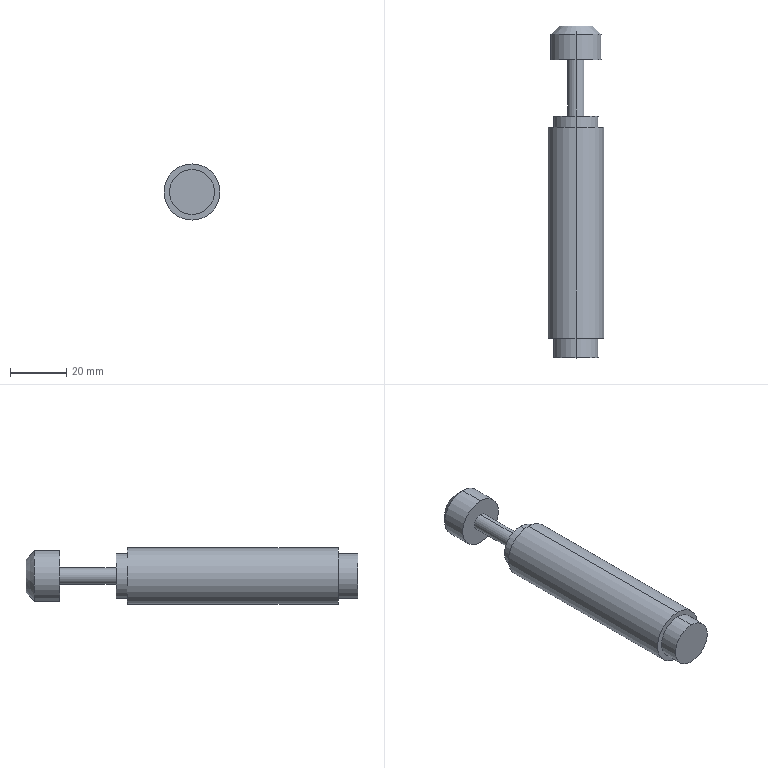Part | STEP file | PN_0009 (hydraulic changer ACA2020) | 1 solid | 18 faces | box 20 x 118 x 20 mm | volume 29167 mm3 | cylinder 10 | plane 6 | cone 2 | commonest cylinder face diameters 16 x4 6 x2 18 x2 20 x2
STEP:
#1=CARTESIAN_POINT('',(0.,0.,0.));
#2=DIRECTION('',(0.,0.,1.));
#3=DIRECTION('',(1.,0.,0.));
#4=AXIS2_PLACEMENT_3D('',#1,#2,#3);
#5=CARTESIAN_POINT('',(0.,118.,6.));
#6=VERTEX_POINT('',#5);
#7=CARTESIAN_POINT('',(0.,118.,-6.));
#8=VERTEX_POINT('',#7);
#9=CARTESIAN_POINT('',(0.,118.,0.));
#10=DIRECTION('',(0.,1.,0.));
#11=DIRECTION('',(0.,0.,1.));
#12=AXIS2_PLACEMENT_3D('',#9,#10,#11);
#13=CIRCLE('',#12,6.);
#14=CARTESIAN_POINT('',(0.,115.,0.));
#15=DIRECTION('',(0.,-1.,0.));
#16=DIRECTION('',(0.,0.,-1.));
#17=AXIS2_PLACEMENT_3D('',#14,#15,#16);
#18=CONICAL_SURFACE('',#17,9.,0.7854);
#19=CARTESIAN_POINT('',(3.142,-3.));
#20=DIRECTION('',(-1.,0.));
#21=VECTOR('',#20,1.);
#22=LINE('',#19,#21);
#23=(GEOMETRIC_REPRESENTATION_CONTEXT(2)PARAMETRIC_REPRESENTATION_CONTEXT()REPRESENTATION_CONTEXT('',''));
#24=DEFINITIONAL_REPRESENTATION('',(#22),#23);
#25=PCURVE('',#18,#24);
#26=CARTESIAN_POINT('',(9.,118.,0.));
#27=DIRECTION('',(0.,1.,0.));
#28=DIRECTION('',(0.,0.,1.));
#29=AXIS2_PLACEMENT_3D('',#26,#27,#28);
#30=PLANE('',#29);
#31=CARTESIAN_POINT('',(0.,-9.));
#32=DIRECTION('',(1.,0.));
#33=AXIS2_PLACEMENT_2D('',#31,#32);
#34=CIRCLE('',#33,6.);
#35=(GEOMETRIC_REPRESENTATION_CONTEXT(2)PARAMETRIC_REPRESENTATION_CONTEXT()REPRESENTATION_CONTEXT('',''));
#36=DEFINITIONAL_REPRESENTATION('',(#34),#35);
#37=PCURVE('',#30,#36);
#38=SURFACE_CURVE('',#13,(#25,#37),.PCURVE_S1.);
#39=EDGE_CURVE('',#6,#8,#38,.T.);
#40=ORIENTED_EDGE('',*,*,#39,.F.);
#41=CARTESIAN_POINT('',(0.,115.,9.));
#42=VERTEX_POINT('',#41);
#43=CARTESIAN_POINT('',(0.,115.,9.));
#44=DIRECTION('',(0.,-0.7071,0.7071));
#45=VECTOR('',#44,1.);
#46=LINE('',#43,#45);
#47=CARTESIAN_POINT('',(3.142,0.));
#48=DIRECTION('',(0.,1.));
#49=VECTOR('',#48,1.);
#50=LINE('',#47,#49);
#51=(GEOMETRIC_REPRESENTATION_CONTEXT(2)PARAMETRIC_REPRESENTATION_CONTEXT()REPRESENTATION_CONTEXT('',''));
#52=DEFINITIONAL_REPRESENTATION('',(#50),#51);
#53=PCURVE('',#18,#52);
#54=CARTESIAN_POINT('',(0.,115.,0.));
#55=DIRECTION('',(0.,-1.,0.));
#56=DIRECTION('',(0.,0.,-1.));
#57=AXIS2_PLACEMENT_3D('',#54,#55,#56);
#58=CONICAL_SURFACE('',#57,9.,0.7854);
#59=CARTESIAN_POINT('',(3.142,0.));
#60=DIRECTION('',(0.,1.));
#61=VECTOR('',#60,1.);
#62=LINE('',#59,#61);
#63=(GEOMETRIC_REPRESENTATION_CONTEXT(2)PARAMETRIC_REPRESENTATION_CONTEXT()REPRESENTATION_CONTEXT('',''));
#64=DEFINITIONAL_REPRESENTATION('',(#62),#63);
#65=PCURVE('',#58,#64);
#66=SURFACE_CURVE('',#46,(#53,#65),.PCURVE_S1.);
#67=EDGE_CURVE('',#6,#42,#66,.T.);
#68=ORIENTED_EDGE('',*,*,#67,.T.);
#69=CARTESIAN_POINT('',(0.,115.,-9.));
#70=VERTEX_POINT('',#69);
#71=CARTESIAN_POINT('',(0.,115.,0.));
#72=DIRECTION('',(0.,-1.,0.));
#73=DIRECTION('',(0.,0.,1.));
#74=AXIS2_PLACEMENT_3D('',#71,#72,#73);
#75=CIRCLE('',#74,9.);
#76=CARTESIAN_POINT('',(-3.142,0.));
#77=DIRECTION('',(1.,0.));
#78=VECTOR('',#77,1.);
#79=LINE('',#76,#78);
#80=(GEOMETRIC_REPRESENTATION_CONTEXT(2)PARAMETRIC_REPRESENTATION_CONTEXT()REPRESENTATION_CONTEXT('',''));
#81=DEFINITIONAL_REPRESENTATION('',(#79),#80);
#82=PCURVE('',#18,#81);
#83=CARTESIAN_POINT('',(0.,0.,0.));
#84=DIRECTION('',(0.,-1.,0.));
#85=DIRECTION('',(0.,0.,-1.));
#86=AXIS2_PLACEMENT_3D('',#83,#84,#85);
#87=CYLINDRICAL_SURFACE('',#86,9.);
#88=CARTESIAN_POINT('',(-3.142,-115.));
#89=DIRECTION('',(1.,0.));
#90=VECTOR('',#89,1.);
#91=LINE('',#88,#90);
#92=(GEOMETRIC_REPRESENTATION_CONTEXT(2)PARAMETRIC_REPRESENTATION_CONTEXT()REPRESENTATION_CONTEXT('',''));
#93=DEFINITIONAL_REPRESENTATION('',(#91),#92);
#94=PCURVE('',#87,#93);
#95=SURFACE_CURVE('',#75,(#82,#94),.PCURVE_S1.);
#96=EDGE_CURVE('',#70,#42,#95,.T.);
#97=ORIENTED_EDGE('',*,*,#96,.F.);
#98=CARTESIAN_POINT('',(0.,115.,-9.));
#99=DIRECTION('',(0.,-0.7071,-0.7071));
#100=VECTOR('',#99,1.);
#101=LINE('',#98,#100);
#102=CARTESIAN_POINT('',(0.,0.));
#103=DIRECTION('',(0.,1.));
#104=VECTOR('',#103,1.);
#105=LINE('',#102,#104);
#106=(GEOMETRIC_REPRESENTATION_CONTEXT(2)PARAMETRIC_REPRESENTATION_CONTEXT()REPRESENTATION_CONTEXT('',''));
#107=DEFINITIONAL_REPRESENTATION('',(#105),#106);
#108=PCURVE('',#18,#107);
#109=CARTESIAN_POINT('',(6.283,0.));
#110=DIRECTION('',(0.,1.));
#111=VECTOR('',#110,1.);
#112=LINE('',#109,#111);
#113=(GEOMETRIC_REPRESENTATION_CONTEXT(2)PARAMETRIC_REPRESENTATION_CONTEXT()REPRESENTATION_CONTEXT('',''));
#114=DEFINITIONAL_REPRESENTATION('',(#112),#113);
#115=PCURVE('',#58,#114);
#116=SURFACE_CURVE('',#101,(#108,#115),.PCURVE_S1.);
#117=EDGE_CURVE('',#8,#70,#116,.T.);
#118=ORIENTED_EDGE('',*,*,#117,.F.);
#119=EDGE_LOOP('',(#40,#68,#97,#118));
#120=FACE_BOUND('',#119,.T.);
#121=ADVANCED_FACE('',(#120),#18,.T.);
#122=ORIENTED_EDGE('',*,*,#96,.T.);
#123=CARTESIAN_POINT('',(0.,106.,9.));
#124=VERTEX_POINT('',#123);
#125=CARTESIAN_POINT('',(0.,0.,9.));
#126=DIRECTION('',(0.,-1.,0.));
#127=VECTOR('',#126,1.);
#128=LINE('',#125,#127);
#129=CARTESIAN_POINT('',(3.142,0.));
#130=DIRECTION('',(0.,1.));
#131=VECTOR('',#130,1.);
#132=LINE('',#129,#131);
#133=(GEOMETRIC_REPRESENTATION_CONTEXT(2)PARAMETRIC_REPRESENTATION_CONTEXT()REPRESENTATION_CONTEXT('',''));
#134=DEFINITIONAL_REPRESENTATION('',(#132),#133);
#135=PCURVE('',#87,#134);
#136=CARTESIAN_POINT('',(0.,0.,0.));
#137=DIRECTION('',(0.,-1.,0.));
#138=DIRECTION('',(0.,0.,-1.));
#139=AXIS2_PLACEMENT_3D('',#136,#137,#138);
#140=CYLINDRICAL_SURFACE('',#139,9.);
#141=CARTESIAN_POINT('',(3.142,0.));
#142=DIRECTION('',(0.,1.));
#143=VECTOR('',#142,1.);
#144=LINE('',#141,#143);
#145=(GEOMETRIC_REPRESENTATION_CONTEXT(2)PARAMETRIC_REPRESENTATION_CONTEXT()REPRESENTATION_CONTEXT('',''));
#146=DEFINITIONAL_REPRESENTATION('',(#144),#145);
#147=PCURVE('',#140,#146);
#148=SURFACE_CURVE('',#128,(#135,#147),.PCURVE_S1.);
#149=EDGE_CURVE('',#42,#124,#148,.T.);
#150=ORIENTED_EDGE('',*,*,#149,.T.);
#151=CARTESIAN_POINT('',(0.,106.,-9.));
#152=VERTEX_POINT('',#151);
#153=CARTESIAN_POINT('',(0.,106.,0.));
#154=DIRECTION('',(0.,-1.,0.));
#155=DIRECTION('',(0.,0.,-1.));
#156=AXIS2_PLACEMENT_3D('',#153,#154,#155);
#157=CIRCLE('',#156,9.);
#158=CARTESIAN_POINT('',(0.,-106.));
#159=DIRECTION('',(1.,0.));
#160=VECTOR('',#159,1.);
#161=LINE('',#158,#160);
#162=(GEOMETRIC_REPRESENTATION_CONTEXT(2)PARAMETRIC_REPRESENTATION_CONTEXT()REPRESENTATION_CONTEXT('',''));
#163=DEFINITIONAL_REPRESENTATION('',(#161),#162);
#164=PCURVE('',#87,#163);
#165=CARTESIAN_POINT('',(3.,106.,0.));
#166=DIRECTION('',(0.,-1.,0.));
#167=DIRECTION('',(0.,0.,-1.));
#168=AXIS2_PLACEMENT_3D('',#165,#166,#167);
#169=PLANE('',#168);
#170=CARTESIAN_POINT('',(0.,-3.));
#171=DIRECTION('',(1.,0.));
#172=AXIS2_PLACEMENT_2D('',#170,#171);
#173=CIRCLE('',#172,9.);
#174=(GEOMETRIC_REPRESENTATION_CONTEXT(2)PARAMETRIC_REPRESENTATION_CONTEXT()REPRESENTATION_CONTEXT('',''));
#175=DEFINITIONAL_REPRESENTATION('',(#173),#174);
#176=PCURVE('',#169,#175);
#177=SURFACE_CURVE('',#157,(#164,#176),.PCURVE_S1.);
#178=EDGE_CURVE('',#152,#124,#177,.T.);
#179=ORIENTED_EDGE('',*,*,#178,.F.);
#180=CARTESIAN_POINT('',(0.,0.,-9.));
#181=DIRECTION('',(0.,-1.,0.));
#182=VECTOR('',#181,1.);
#183=LINE('',#180,#182);
#184=CARTESIAN_POINT('',(0.,0.));
#185=DIRECTION('',(0.,1.));
#186=VECTOR('',#185,1.);
#187=LINE('',#184,#186);
#188=(GEOMETRIC_REPRESENTATION_CONTEXT(2)PARAMETRIC_REPRESENTATION_CONTEXT()REPRESENTATION_CONTEXT('',''));
#189=DEFINITIONAL_REPRESENTATION('',(#187),#188);
#190=PCURVE('',#87,#189);
#191=CARTESIAN_POINT('',(6.283,0.));
#192=DIRECTION('',(0.,1.));
#193=VECTOR('',#192,1.);
#194=LINE('',#191,#193);
#195=(GEOMETRIC_REPRESENTATION_CONTEXT(2)PARAMETRIC_REPRESENTATION_CONTEXT()REPRESENTATION_CONTEXT('',''));
#196=DEFINITIONAL_REPRESENTATION('',(#194),#195);
#197=PCURVE('',#140,#196);
#198=SURFACE_CURVE('',#183,(#190,#197),.PCURVE_S1.);
#199=EDGE_CURVE('',#70,#152,#198,.T.);
#200=ORIENTED_EDGE('',*,*,#199,.F.);
#201=EDGE_LOOP('',(#122,#150,#179,#200));
#202=FACE_BOUND('',#201,.T.);
#203=ADVANCED_FACE('',(#202),#87,.T.);
#204=CARTESIAN_POINT('',(0.,106.,-3.));
#205=VERTEX_POINT('',#204);
#206=CARTESIAN_POINT('',(0.,106.,3.));
#207=VERTEX_POINT('',#206);
#208=CARTESIAN_POINT('',(0.,106.,0.));
#209=DIRECTION('',(0.,-1.,0.));
#210=DIRECTION('',(0.,0.,-1.));
#211=AXIS2_PLACEMENT_3D('',#208,#209,#210);
#212=CIRCLE('',#211,3.);
#213=CARTESIAN_POINT('',(0.,0.,0.));
#214=DIRECTION('',(0.,-1.,0.));
#215=DIRECTION('',(0.,0.,-1.));
#216=AXIS2_PLACEMENT_3D('',#213,#214,#215);
#217=CYLINDRICAL_SURFACE('',#216,3.);
#218=CARTESIAN_POINT('',(0.,-106.));
#219=DIRECTION('',(1.,0.));
#220=VECTOR('',#219,1.);
#221=LINE('',#218,#220);
#222=(GEOMETRIC_REPRESENTATION_CONTEXT(2)PARAMETRIC_REPRESENTATION_CONTEXT()REPRESENTATION_CONTEXT('',''));
#223=DEFINITIONAL_REPRESENTATION('',(#221),#222);
#224=PCURVE('',#217,#223);
#225=CARTESIAN_POINT('',(0.,-3.));
#226=DIRECTION('',(1.,0.));
#227=AXIS2_PLACEMENT_2D('',#225,#226);
#228=CIRCLE('',#227,3.);
#229=(GEOMETRIC_REPRESENTATION_CONTEXT(2)PARAMETRIC_REPRESENTATION_CONTEXT()REPRESENTATION_CONTEXT('',''));
#230=DEFINITIONAL_REPRESENTATION('',(#228),#229);
#231=PCURVE('',#169,#230);
#232=SURFACE_CURVE('',#212,(#224,#231),.PCURVE_S1.);
#233=EDGE_CURVE('',#205,#207,#232,.T.);
#234=ORIENTED_EDGE('',*,*,#233,.T.);
#235=CARTESIAN_POINT('',(0.,86.,3.));
#236=VERTEX_POINT('',#235);
#237=CARTESIAN_POINT('',(0.,0.,3.));
#238=DIRECTION('',(0.,-1.,0.));
#239=VECTOR('',#238,1.);
#240=LINE('',#237,#239);
#241=CARTESIAN_POINT('',(3.142,0.));
#242=DIRECTION('',(0.,1.));
#243=VECTOR('',#242,1.);
#244=LINE('',#241,#243);
#245=(GEOMETRIC_REPRESENTATION_CONTEXT(2)PARAMETRIC_REPRESENTATION_CONTEXT()REPRESENTATION_CONTEXT('',''));
#246=DEFINITIONAL_REPRESENTATION('',(#244),#245);
#247=PCURVE('',#217,#246);
#248=CARTESIAN_POINT('',(0.,0.,0.));
#249=DIRECTION('',(0.,-1.,0.));
#250=DIRECTION('',(0.,0.,-1.));
#251=AXIS2_PLACEMENT_3D('',#248,#249,#250);
#252=CYLINDRICAL_SURFACE('',#251,3.);
#253=CARTESIAN_POINT('',(3.142,0.));
#254=DIRECTION('',(0.,1.));
#255=VECTOR('',#254,1.);
#256=LINE('',#253,#255);
#257=(GEOMETRIC_REPRESENTATION_CONTEXT(2)PARAMETRIC_REPRESENTATION_CONTEXT()REPRESENTATION_CONTEXT('',''));
#258=DEFINITIONAL_REPRESENTATION('',(#256),#257);
#259=PCURVE('',#252,#258);
#260=SURFACE_CURVE('',#240,(#247,#259),.PCURVE_S1.);
#261=EDGE_CURVE('',#207,#236,#260,.T.);
#262=ORIENTED_EDGE('',*,*,#261,.T.);
#263=CARTESIAN_POINT('',(0.,86.,-3.));
#264=VERTEX_POINT('',#263);
#265=CARTESIAN_POINT('',(0.,86.,0.));
#266=DIRECTION('',(0.,-1.,0.));
#267=DIRECTION('',(0.,0.,-1.));
#268=AXIS2_PLACEMENT_3D('',#265,#266,#267);
#269=CIRCLE('',#268,3.);
#270=CARTESIAN_POINT('',(0.,-86.));
#271=DIRECTION('',(1.,0.));
#272=VECTOR('',#271,1.);
#273=LINE('',#270,#272);
#274=(GEOMETRIC_REPRESENTATION_CONTEXT(2)PARAMETRIC_REPRESENTATION_CONTEXT()REPRESENTATION_CONTEXT('',''));
#275=DEFINITIONAL_REPRESENTATION('',(#273),#274);
#276=PCURVE('',#217,#275);
#277=CARTESIAN_POINT('',(8.,86.,0.));
#278=DIRECTION('',(0.,1.,0.));
#279=DIRECTION('',(0.,0.,1.));
#280=AXIS2_PLACEMENT_3D('',#277,#278,#279);
#281=PLANE('',#280);
#282=CARTESIAN_POINT('',(-3.,-8.));
#283=CARTESIAN_POINT('',(-3.,-2.804));
#284=CARTESIAN_POINT('',(1.5,-5.402));
#285=CARTESIAN_POINT('',(6.,-8.));
#286=CARTESIAN_POINT('',(1.5,-10.598));
#287=CARTESIAN_POINT('',(-3.,-13.196));
#288=CARTESIAN_POINT('',(-3.,-8.));
#289=(BOUNDED_CURVE()B_SPLINE_CURVE(2,(#282,#283,#284,#285,#286,#287,#288),.UNSPECIFIED.,.T.,.F.)B_SPLINE_CURVE_WITH_KNOTS((1,2,2,2,2,1),(-2.094,0.,2.094,4.189,6.283,8.378),.UNSPECIFIED.)CURVE()GEOMETRIC_REPRESENTATION_ITEM()RATIONAL_B_SPLINE_CURVE((1.,0.5,1.,0.5,1.,0.5,1.))REPRESENTATION_ITEM(''));
#290=(GEOMETRIC_REPRESENTATION_CONTEXT(2)PARAMETRIC_REPRESENTATION_CONTEXT()REPRESENTATION_CONTEXT('',''));
#291=DEFINITIONAL_REPRESENTATION('',(#289),#290);
#292=PCURVE('',#281,#291);
#293=SURFACE_CURVE('',#269,(#276,#292),.PCURVE_S1.);
#294=EDGE_CURVE('',#264,#236,#293,.T.);
#295=ORIENTED_EDGE('',*,*,#294,.F.);
#296=CARTESIAN_POINT('',(0.,0.,-3.));
#297=DIRECTION('',(0.,-1.,0.));
#298=VECTOR('',#297,1.);
#299=LINE('',#296,#298);
#300=CARTESIAN_POINT('',(0.,0.));
#301=DIRECTION('',(0.,1.));
#302=VECTOR('',#301,1.);
#303=LINE('',#300,#302);
#304=(GEOMETRIC_REPRESENTATION_CONTEXT(2)PARAMETRIC_REPRESENTATION_CONTEXT()REPRESENTATION_CONTEXT('',''));
#305=DEFINITIONAL_REPRESENTATION('',(#303),#304);
#306=PCURVE('',#217,#305);
#307=CARTESIAN_POINT('',(6.283,0.));
#308=DIRECTION('',(0.,1.));
#309=VECTOR('',#308,1.);
#310=LINE('',#307,#309);
#311=(GEOMETRIC_REPRESENTATION_CONTEXT(2)PARAMETRIC_REPRESENTATION_CONTEXT()REPRESENTATION_CONTEXT('',''));
#312=DEFINITIONAL_REPRESENTATION('',(#310),#311);
#313=PCURVE('',#252,#312);
#314=SURFACE_CURVE('',#299,(#306,#313),.PCURVE_S1.);
#315=EDGE_CURVE('',#205,#264,#314,.T.);
#316=ORIENTED_EDGE('',*,*,#315,.F.);
#317=EDGE_LOOP('',(#234,#262,#295,#316));
#318=FACE_BOUND('',#317,.T.);
#319=ADVANCED_FACE('',(#318),#217,.T.);
#320=CARTESIAN_POINT('',(0.,86.,-8.));
#321=VERTEX_POINT('',#320);
#322=CARTESIAN_POINT('',(0.,86.,8.));
#323=VERTEX_POINT('',#322);
#324=CARTESIAN_POINT('',(0.,86.,0.));
#325=DIRECTION('',(0.,-1.,0.));
#326=DIRECTION('',(0.,0.,-1.));
#327=AXIS2_PLACEMENT_3D('',#324,#325,#326);
#328=CIRCLE('',#327,8.);
#329=CARTESIAN_POINT('',(0.,0.,0.));
#330=DIRECTION('',(0.,-1.,0.));
#331=DIRECTION('',(0.,0.,-1.));
#332=AXIS2_PLACEMENT_3D('',#329,#330,#331);
#333=CYLINDRICAL_SURFACE('',#332,8.);
#334=CARTESIAN_POINT('',(0.,-86.));
#335=DIRECTION('',(1.,0.));
#336=VECTOR('',#335,1.);
#337=LINE('',#334,#336);
#338=(GEOMETRIC_REPRESENTATION_CONTEXT(2)PARAMETRIC_REPRESENTATION_CONTEXT()REPRESENTATION_CONTEXT('',''));
#339=DEFINITIONAL_REPRESENTATION('',(#337),#338);
#340=PCURVE('',#333,#339);
#341=CARTESIAN_POINT('',(-8.,-8.));
#342=CARTESIAN_POINT('',(-8.,5.856));
#343=CARTESIAN_POINT('',(4.,-1.072));
#344=CARTESIAN_POINT('',(16.,-8.));
#345=CARTESIAN_POINT('',(4.,-14.928));
#346=CARTESIAN_POINT('',(-8.,-21.856));
#347=CARTESIAN_POINT('',(-8.,-8.));
#348=(BOUNDED_CURVE()B_SPLINE_CURVE(2,(#341,#342,#343,#344,#345,#346,#347),.UNSPECIFIED.,.T.,.F.)B_SPLINE_CURVE_WITH_KNOTS((1,2,2,2,2,1),(-2.094,0.,2.094,4.189,6.283,8.378),.UNSPECIFIED.)CURVE()GEOMETRIC_REPRESENTATION_ITEM()RATIONAL_B_SPLINE_CURVE((1.,0.5,1.,0.5,1.,0.5,1.))REPRESENTATION_ITEM(''));
#349=(GEOMETRIC_REPRESENTATION_CONTEXT(2)PARAMETRIC_REPRESENTATION_CONTEXT()REPRESENTATION_CONTEXT('',''));
#350=DEFINITIONAL_REPRESENTATION('',(#348),#349);
#351=PCURVE('',#281,#350);
#352=SURFACE_CURVE('',#328,(#340,#351),.PCURVE_S1.);
#353=EDGE_CURVE('',#321,#323,#352,.T.);
#354=ORIENTED_EDGE('',*,*,#353,.T.);
#355=CARTESIAN_POINT('',(0.,82.,8.));
#356=VERTEX_POINT('',#355);
#357=CARTESIAN_POINT('',(0.,0.,8.));
#358=DIRECTION('',(0.,-1.,0.));
#359=VECTOR('',#358,1.);
#360=LINE('',#357,#359);
#361=CARTESIAN_POINT('',(3.142,0.));
#362=DIRECTION('',(0.,1.));
#363=VECTOR('',#362,1.);
#364=LINE('',#361,#363);
#365=(GEOMETRIC_REPRESENTATION_CONTEXT(2)PARAMETRIC_REPRESENTATION_CONTEXT()REPRESENTATION_CONTEXT('',''));
#366=DEFINITIONAL_REPRESENTATION('',(#364),#365);
#367=PCURVE('',#333,#366);
#368=CARTESIAN_POINT('',(0.,0.,0.));
#369=DIRECTION('',(0.,-1.,0.));
#370=DIRECTION('',(0.,0.,-1.));
#371=AXIS2_PLACEMENT_3D('',#368,#369,#370);
#372=CYLINDRICAL_SURFACE('',#371,8.);
#373=CARTESIAN_POINT('',(3.142,0.));
#374=DIRECTION('',(0.,1.));
#375=VECTOR('',#374,1.);
#376=LINE('',#373,#375);
#377=(GEOMETRIC_REPRESENTATION_CONTEXT(2)PARAMETRIC_REPRESENTATION_CONTEXT()REPRESENTATION_CONTEXT('',''));
#378=DEFINITIONAL_REPRESENTATION('',(#376),#377);
#379=PCURVE('',#372,#378);
#380=SURFACE_CURVE('',#360,(#367,#379),.PCURVE_S1.);
#381=EDGE_CURVE('',#323,#356,#380,.T.);
#382=ORIENTED_EDGE('',*,*,#381,.T.);
#383=CARTESIAN_POINT('',(0.,82.,-8.));
#384=VERTEX_POINT('',#383);
#385=CARTESIAN_POINT('',(0.,82.,0.));
#386=DIRECTION('',(0.,-1.,0.));
#387=DIRECTION('',(0.,0.,-1.));
#388=AXIS2_PLACEMENT_3D('',#385,#386,#387);
#389=CIRCLE('',#388,8.);
#390=CARTESIAN_POINT('',(0.,-82.));
#391=DIRECTION('',(1.,0.));
#392=VECTOR('',#391,1.);
#393=LINE('',#390,#392);
#394=(GEOMETRIC_REPRESENTATION_CONTEXT(2)PARAMETRIC_REPRESENTATION_CONTEXT()REPRESENTATION_CONTEXT('',''));
#395=DEFINITIONAL_REPRESENTATION('',(#393),#394);
#396=PCURVE('',#333,#395);
#397=CARTESIAN_POINT('',(10.,82.,0.));
#398=DIRECTION('',(0.,1.,0.));
#399=DIRECTION('',(0.,0.,1.));
#400=AXIS2_PLACEMENT_3D('',#397,#398,#399);
#401=PLANE('',#400);
#402=CARTESIAN_POINT('',(-8.,-10.));
#403=CARTESIAN_POINT('',(-8.,3.856));
#404=CARTESIAN_POINT('',(4.,-3.072));
#405=CARTESIAN_POINT('',(16.,-10.));
#406=CARTESIAN_POINT('',(4.,-16.928));
#407=CARTESIAN_POINT('',(-8.,-23.856));
#408=CARTESIAN_POINT('',(-8.,-10.));
#409=(BOUNDED_CURVE()B_SPLINE_CURVE(2,(#402,#403,#404,#405,#406,#407,#408),.UNSPECIFIED.,.T.,.F.)B_SPLINE_CURVE_WITH_KNOTS((1,2,2,2,2,1),(-2.094,0.,2.094,4.189,6.283,8.378),.UNSPECIFIED.)CURVE()GEOMETRIC_REPRESENTATION_ITEM()RATIONAL_B_SPLINE_CURVE((1.,0.5,1.,0.5,1.,0.5,1.))REPRESENTATION_ITEM(''));
#410=(GEOMETRIC_REPRESENTATION_CONTEXT(2)PARAMETRIC_REPRESENTATION_CONTEXT()REPRESENTATION_CONTEXT('',''));
#411=DEFINITIONAL_REPRESENTATION('',(#409),#410);
#412=PCURVE('',#401,#411);
#413=SURFACE_CURVE('',#389,(#396,#412),.PCURVE_S1.);
#414=EDGE_CURVE('',#384,#356,#413,.T.);
#415=ORIENTED_EDGE('',*,*,#414,.F.);
#416=CARTESIAN_POINT('',(0.,0.,-8.));
#417=DIRECTION('',(0.,-1.,0.));
#418=VECTOR('',#417,1.);
#419=LINE('',#416,#418);
#420=CARTESIAN_POINT('',(0.,0.));
#421=DIRECTION('',(0.,1.));
#422=VECTOR('',#421,1.);
#423=LINE('',#420,#422);
#424=(GEOMETRIC_REPRESENTATION_CONTEXT(2)PARAMETRIC_REPRESENTATION_CONTEXT()REPRESENTATION_CONTEXT('',''));
#425=DEFINITIONAL_REPRESENTATION('',(#423),#424);
#426=PCURVE('',#333,#425);
#427=CARTESIAN_POINT('',(6.283,0.));
#428=DIRECTION('',(0.,1.));
#429=VECTOR('',#428,1.);
#430=LINE('',#427,#429);
#431=(GEOMETRIC_REPRESENTATION_CONTEXT(2)PARAMETRIC_REPRESENTATION_CONTEXT()REPRESENTATION_CONTEXT('',''));
#432=DEFINITIONAL_REPRESENTATION('',(#430),#431);
#433=PCURVE('',#372,#432);
#434=SURFACE_CURVE('',#419,(#426,#433),.PCURVE_S1.);
#435=EDGE_CURVE('',#321,#384,#434,.T.);
#436=ORIENTED_EDGE('',*,*,#435,.F.);
#437=EDGE_LOOP('',(#354,#382,#415,#436));
#438=FACE_BOUND('',#437,.T.);
#439=ADVANCED_FACE('',(#438),#333,.T.);
#440=CARTESIAN_POINT('',(0.,82.,-10.));
#441=VERTEX_POINT('',#440);
#442=CARTESIAN_POINT('',(0.,82.,10.));
#443=VERTEX_POINT('',#442);
#444=CARTESIAN_POINT('',(0.,82.,0.));
#445=DIRECTION('',(0.,-1.,0.));
#446=DIRECTION('',(0.,0.,-1.));
#447=AXIS2_PLACEMENT_3D('',#444,#445,#446);
#448=CIRCLE('',#447,10.);
#449=CARTESIAN_POINT('',(0.,0.,0.));
#450=DIRECTION('',(0.,-1.,0.));
#451=DIRECTION('',(0.,0.,-1.));
#452=AXIS2_PLACEMENT_3D('',#449,#450,#451);
#453=CYLINDRICAL_SURFACE('',#452,10.);
#454=CARTESIAN_POINT('',(0.,-82.));
#455=DIRECTION('',(1.,0.));
#456=VECTOR('',#455,1.);
#457=LINE('',#454,#456);
#458=(GEOMETRIC_REPRESENTATION_CONTEXT(2)PARAMETRIC_REPRESENTATION_CONTEXT()REPRESENTATION_CONTEXT('',''));
#459=DEFINITIONAL_REPRESENTATION('',(#457),#458);
#460=PCURVE('',#453,#459);
#461=CARTESIAN_POINT('',(-10.,-10.));
#462=CARTESIAN_POINT('',(-10.,7.321));
#463=CARTESIAN_POINT('',(5.,-1.34));
#464=CARTESIAN_POINT('',(20.,-10.));
#465=CARTESIAN_POINT('',(5.,-18.66));
#466=CARTESIAN_POINT('',(-10.,-27.321));
#467=CARTESIAN_POINT('',(-10.,-10.));
#468=(BOUNDED_CURVE()B_SPLINE_CURVE(2,(#461,#462,#463,#464,#465,#466,#467),.UNSPECIFIED.,.T.,.F.)B_SPLINE_CURVE_WITH_KNOTS((1,2,2,2,2,1),(-2.094,0.,2.094,4.189,6.283,8.378),.UNSPECIFIED.)CURVE()GEOMETRIC_REPRESENTATION_ITEM()RATIONAL_B_SPLINE_CURVE((1.,0.5,1.,0.5,1.,0.5,1.))REPRESENTATION_ITEM(''));
#469=(GEOMETRIC_REPRESENTATION_CONTEXT(2)PARAMETRIC_REPRESENTATION_CONTEXT()REPRESENTATION_CONTEXT('',''));
#470=DEFINITIONAL_REPRESENTATION('',(#468),#469);
#471=PCURVE('',#401,#470);
#472=SURFACE_CURVE('',#448,(#460,#471),.PCURVE_S1.);
#473=EDGE_CURVE('',#441,#443,#472,.T.);
#474=ORIENTED_EDGE('',*,*,#473,.T.);
#475=CARTESIAN_POINT('',(0.,7.,10.));
#476=VERTEX_POINT('',#475);
#477=CARTESIAN_POINT('',(0.,0.,10.));
#478=DIRECTION('',(0.,-1.,0.));
#479=VECTOR('',#478,1.);
#480=LINE('',#477,#479);
#481=CARTESIAN_POINT('',(3.142,0.));
#482=DIRECTION('',(0.,1.));
#483=VECTOR('',#482,1.);
#484=LINE('',#481,#483);
#485=(GEOMETRIC_REPRESENTATION_CONTEXT(2)PARAMETRIC_REPRESENTATION_CONTEXT()REPRESENTATION_CONTEXT('',''));
#486=DEFINITIONAL_REPRESENTATION('',(#484),#485);
#487=PCURVE('',#453,#486);
#488=CARTESIAN_POINT('',(0.,0.,0.));
#489=DIRECTION('',(0.,-1.,0.));
#490=DIRECTION('',(0.,0.,-1.));
#491=AXIS2_PLACEMENT_3D('',#488,#489,#490);
#492=CYLINDRICAL_SURFACE('',#491,10.);
#493=CARTESIAN_POINT('',(3.142,0.));
#494=DIRECTION('',(0.,1.));
#495=VECTOR('',#494,1.);
#496=LINE('',#493,#495);
#497=(GEOMETRIC_REPRESENTATION_CONTEXT(2)PARAMETRIC_REPRESENTATION_CONTEXT()REPRESENTATION_CONTEXT('',''));
#498=DEFINITIONAL_REPRESENTATION('',(#496),#497);
#499=PCURVE('',#492,#498);
#500=SURFACE_CURVE('',#480,(#487,#499),.PCURVE_S1.);
#501=EDGE_CURVE('',#443,#476,#500,.T.);
#502=ORIENTED_EDGE('',*,*,#501,.T.);
#503=CARTESIAN_POINT('',(0.,7.,-10.));
#504=VERTEX_POINT('',#503);
#505=CARTESIAN_POINT('',(0.,7.,0.));
#506=DIRECTION('',(0.,-1.,0.));
#507=DIRECTION('',(0.,0.,-1.));
#508=AXIS2_PLACEMENT_3D('',#505,#506,#507);
#509=CIRCLE('',#508,10.);
#510=CARTESIAN_POINT('',(0.,-7.));
#511=DIRECTION('',(1.,0.));
#512=VECTOR('',#511,1.);
#513=LINE('',#510,#512);
#514=(GEOMETRIC_REPRESENTATION_CONTEXT(2)PARAMETRIC_REPRESENTATION_CONTEXT()REPRESENTATION_CONTEXT('',''));
#515=DEFINITIONAL_REPRESENTATION('',(#513),#514);
#516=PCURVE('',#453,#515);
#517=CARTESIAN_POINT('',(8.,7.,0.));
#518=DIRECTION('',(0.,-1.,0.));
#519=DIRECTION('',(0.,0.,-1.));
#520=AXIS2_PLACEMENT_3D('',#517,#518,#519);
#521=PLANE('',#520);
#522=CARTESIAN_POINT('',(0.,-8.));
#523=DIRECTION('',(1.,0.));
#524=AXIS2_PLACEMENT_2D('',#522,#523);
#525=CIRCLE('',#524,10.);
#526=(GEOMETRIC_REPRESENTATION_CONTEXT(2)PARAMETRIC_REPRESENTATION_CONTEXT()REPRESENTATION_CONTEXT('',''));
#527=DEFINITIONAL_REPRESENTATION('',(#525),#526);
#528=PCURVE('',#521,#527);
#529=SURFACE_CURVE('',#509,(#516,#528),.PCURVE_S1.);
#530=EDGE_CURVE('',#504,#476,#529,.T.);
#531=ORIENTED_EDGE('',*,*,#530,.F.);
#532=CARTESIAN_POINT('',(0.,0.,-10.));
#533=DIRECTION('',(0.,-1.,0.));
#534=VECTOR('',#533,1.);
#535=LINE('',#532,#534);
#536=CARTESIAN_POINT('',(0.,0.));
#537=DIRECTION('',(0.,1.));
#538=VECTOR('',#537,1.);
#539=LINE('',#536,#538);
#540=(GEOMETRIC_REPRESENTATION_CONTEXT(2)PARAMETRIC_REPRESENTATION_CONTEXT()REPRESENTATION_CONTEXT('',''));
#541=DEFINITIONAL_REPRESENTATION('',(#539),#540);
#542=PCURVE('',#453,#541);
#543=CARTESIAN_POINT('',(6.283,0.));
#544=DIRECTION('',(0.,1.));
#545=VECTOR('',#544,1.);
#546=LINE('',#543,#545);
#547=(GEOMETRIC_REPRESENTATION_CONTEXT(2)PARAMETRIC_REPRESENTATION_CONTEXT()REPRESENTATION_CONTEXT('',''));
#548=DEFINITIONAL_REPRESENTATION('',(#546),#547);
#549=PCURVE('',#492,#548);
#550=SURFACE_CURVE('',#535,(#542,#549),.PCURVE_S1.);
#551=EDGE_CURVE('',#441,#504,#550,.T.);
#552=ORIENTED_EDGE('',*,*,#551,.F.);
#553=EDGE_LOOP('',(#474,#502,#531,#552));
#554=FACE_BOUND('',#553,.T.);
#555=ADVANCED_FACE('',(#554),#453,.T.);
#556=CARTESIAN_POINT('',(0.,7.,-8.));
#557=VERTEX_POINT('',#556);
#558=CARTESIAN_POINT('',(0.,7.,8.));
#559=VERTEX_POINT('',#558);
#560=CARTESIAN_POINT('',(0.,7.,0.));
#561=DIRECTION('',(0.,-1.,0.));
#562=DIRECTION('',(0.,0.,-1.));
#563=AXIS2_PLACEMENT_3D('',#560,#561,#562);
#564=CIRCLE('',#563,8.);
#565=CARTESIAN_POINT('',(0.,0.,0.));
#566=DIRECTION('',(0.,-1.,0.));
#567=DIRECTION('',(0.,0.,-1.));
#568=AXIS2_PLACEMENT_3D('',#565,#566,#567);
#569=CYLINDRICAL_SURFACE('',#568,8.);
#570=CARTESIAN_POINT('',(0.,-7.));
#571=DIRECTION('',(1.,0.));
#572=VECTOR('',#571,1.);
#573=LINE('',#570,#572);
#574=(GEOMETRIC_REPRESENTATION_CONTEXT(2)PARAMETRIC_REPRESENTATION_CONTEXT()REPRESENTATION_CONTEXT('',''));
#575=DEFINITIONAL_REPRESENTATION('',(#573),#574);
#576=PCURVE('',#569,#575);
#577=CARTESIAN_POINT('',(0.,-8.));
#578=DIRECTION('',(1.,0.));
#579=AXIS2_PLACEMENT_2D('',#577,#578);
#580=CIRCLE('',#579,8.);
#581=(GEOMETRIC_REPRESENTATION_CONTEXT(2)PARAMETRIC_REPRESENTATION_CONTEXT()REPRESENTATION_CONTEXT('',''));
#582=DEFINITIONAL_REPRESENTATION('',(#580),#581);
#583=PCURVE('',#521,#582);
#584=SURFACE_CURVE('',#564,(#576,#583),.PCURVE_S1.);
#585=EDGE_CURVE('',#557,#559,#584,.T.);
#586=ORIENTED_EDGE('',*,*,#585,.T.);
#587=CARTESIAN_POINT('',(0.,0.,8.));
#588=VERTEX_POINT('',#587);
#589=CARTESIAN_POINT('',(0.,0.,8.));
#590=DIRECTION('',(0.,-1.,0.));
#591=VECTOR('',#590,1.);
#592=LINE('',#589,#591);
#593=CARTESIAN_POINT('',(3.142,0.));
#594=DIRECTION('',(0.,1.));
#595=VECTOR('',#594,1.);
#596=LINE('',#593,#595);
#597=(GEOMETRIC_REPRESENTATION_CONTEXT(2)PARAMETRIC_REPRESENTATION_CONTEXT()REPRESENTATION_CONTEXT('',''));
#598=DEFINITIONAL_REPRESENTATION('',(#596),#597);
#599=PCURVE('',#569,#598);
#600=CARTESIAN_POINT('',(0.,0.,0.));
#601=DIRECTION('',(0.,-1.,0.));
#602=DIRECTION('',(0.,0.,-1.));
#603=AXIS2_PLACEMENT_3D('',#600,#601,#602);
#604=CYLINDRICAL_SURFACE('',#603,8.);
#605=CARTESIAN_POINT('',(3.142,0.));
#606=DIRECTION('',(0.,1.));
#607=VECTOR('',#606,1.);
#608=LINE('',#605,#607);
#609=(GEOMETRIC_REPRESENTATION_CONTEXT(2)PARAMETRIC_REPRESENTATION_CONTEXT()REPRESENTATION_CONTEXT('',''));
#610=DEFINITIONAL_REPRESENTATION('',(#608),#609);
#611=PCURVE('',#604,#610);
#612=SURFACE_CURVE('',#592,(#599,#611),.PCURVE_S1.);
#613=EDGE_CURVE('',#559,#588,#612,.T.);
#614=ORIENTED_EDGE('',*,*,#613,.T.);
#615=CARTESIAN_POINT('',(0.,0.,-8.));
#616=VERTEX_POINT('',#615);
#617=CARTESIAN_POINT('',(0.,0.,0.));
#618=DIRECTION('',(0.,-1.,0.));
#619=DIRECTION('',(0.,0.,-1.));
#620=AXIS2_PLACEMENT_3D('',#617,#618,#619);
#621=CIRCLE('',#620,8.);
#622=CARTESIAN_POINT('',(0.,0.));
#623=DIRECTION('',(1.,0.));
#624=VECTOR('',#623,1.);
#625=LINE('',#622,#624);
#626=(GEOMETRIC_REPRESENTATION_CONTEXT(2)PARAMETRIC_REPRESENTATION_CONTEXT()REPRESENTATION_CONTEXT('',''));
#627=DEFINITIONAL_REPRESENTATION('',(#625),#626);
#628=PCURVE('',#569,#627);
#629=CARTESIAN_POINT('',(0.,0.,0.));
#630=DIRECTION('',(0.,-1.,0.));
#631=DIRECTION('',(0.,0.,-1.));
#632=AXIS2_PLACEMENT_3D('',#629,#630,#631);
#633=PLANE('',#632);
#634=CARTESIAN_POINT('',(0.,0.));
#635=DIRECTION('',(1.,0.));
#636=AXIS2_PLACEMENT_2D('',#634,#635);
#637=CIRCLE('',#636,8.);
#638=(GEOMETRIC_REPRESENTATION_CONTEXT(2)PARAMETRIC_REPRESENTATION_CONTEXT()REPRESENTATION_CONTEXT('',''));
#639=DEFINITIONAL_REPRESENTATION('',(#637),#638);
#640=PCURVE('',#633,#639);
#641=SURFACE_CURVE('',#621,(#628,#640),.PCURVE_S1.);
#642=EDGE_CURVE('',#616,#588,#641,.T.);
#643=ORIENTED_EDGE('',*,*,#642,.F.);
#644=CARTESIAN_POINT('',(0.,0.,-8.));
#645=DIRECTION('',(0.,-1.,0.));
#646=VECTOR('',#645,1.);
#647=LINE('',#644,#646);
#648=CARTESIAN_POINT('',(0.,0.));
#649=DIRECTION('',(0.,1.));
#650=VECTOR('',#649,1.);
#651=LINE('',#648,#650);
#652=(GEOMETRIC_REPRESENTATION_CONTEXT(2)PARAMETRIC_REPRESENTATION_CONTEXT()REPRESENTATION_CONTEXT('',''));
#653=DEFINITIONAL_REPRESENTATION('',(#651),#652);
#654=PCURVE('',#569,#653);
#655=CARTESIAN_POINT('',(6.283,0.));
#656=DIRECTION('',(0.,1.));
#657=VECTOR('',#656,1.);
#658=LINE('',#655,#657);
#659=(GEOMETRIC_REPRESENTATION_CONTEXT(2)PARAMETRIC_REPRESENTATION_CONTEXT()REPRESENTATION_CONTEXT('',''));
#660=DEFINITIONAL_REPRESENTATION('',(#658),#659);
#661=PCURVE('',#604,#660);
#662=SURFACE_CURVE('',#647,(#654,#661),.PCURVE_S1.);
#663=EDGE_CURVE('',#557,#616,#662,.T.);
#664=ORIENTED_EDGE('',*,*,#663,.F.);
#665=EDGE_LOOP('',(#586,#614,#643,#664));
#666=FACE_BOUND('',#665,.T.);
#667=ADVANCED_FACE('',(#666),#569,.T.);
#668=ORIENTED_EDGE('',*,*,#642,.T.);
#669=CARTESIAN_POINT('',(0.,0.,0.));
#670=DIRECTION('',(0.,-1.,0.));
#671=DIRECTION('',(0.,0.,-1.));
#672=AXIS2_PLACEMENT_3D('',#669,#670,#671);
#673=CIRCLE('',#672,8.);
#674=CARTESIAN_POINT('',(0.,0.));
#675=DIRECTION('',(1.,0.));
#676=AXIS2_PLACEMENT_2D('',#674,#675);
#677=CIRCLE('',#676,8.);
#678=(GEOMETRIC_REPRESENTATION_CONTEXT(2)PARAMETRIC_REPRESENTATION_CONTEXT()REPRESENTATION_CONTEXT('',''));
#679=DEFINITIONAL_REPRESENTATION('',(#677),#678);
#680=PCURVE('',#633,#679);
#681=CARTESIAN_POINT('',(0.,0.));
#682=DIRECTION('',(1.,0.));
#683=VECTOR('',#682,1.);
#684=LINE('',#681,#683);
#685=(GEOMETRIC_REPRESENTATION_CONTEXT(2)PARAMETRIC_REPRESENTATION_CONTEXT()REPRESENTATION_CONTEXT('',''));
#686=DEFINITIONAL_REPRESENTATION('',(#684),#685);
#687=PCURVE('',#604,#686);
#688=SURFACE_CURVE('',#673,(#680,#687),.PCURVE_S1.);
#689=EDGE_CURVE('',#588,#616,#688,.T.);
#690=ORIENTED_EDGE('',*,*,#689,.T.);
#691=EDGE_LOOP('',(#668,#690));
#692=FACE_BOUND('',#691,.T.);
#693=ADVANCED_FACE('',(#692),#633,.T.);
#694=ORIENTED_EDGE('',*,*,#613,.F.);
#695=CARTESIAN_POINT('',(0.,7.,0.));
#696=DIRECTION('',(0.,-1.,0.));
#697=DIRECTION('',(0.,0.,-1.));
#698=AXIS2_PLACEMENT_3D('',#695,#696,#697);
#699=CIRCLE('',#698,8.);
#700=CARTESIAN_POINT('',(0.,-7.));
#701=DIRECTION('',(1.,0.));
#702=VECTOR('',#701,1.);
#703=LINE('',#700,#702);
#704=(GEOMETRIC_REPRESENTATION_CONTEXT(2)PARAMETRIC_REPRESENTATION_CONTEXT()REPRESENTATION_CONTEXT('',''));
#705=DEFINITIONAL_REPRESENTATION('',(#703),#704);
#706=PCURVE('',#604,#705);
#707=CARTESIAN_POINT('',(0.,-8.));
#708=DIRECTION('',(1.,0.));
#709=AXIS2_PLACEMENT_2D('',#707,#708);
#710=CIRCLE('',#709,8.);
#711=(GEOMETRIC_REPRESENTATION_CONTEXT(2)PARAMETRIC_REPRESENTATION_CONTEXT()REPRESENTATION_CONTEXT('',''));
#712=DEFINITIONAL_REPRESENTATION('',(#710),#711);
#713=PCURVE('',#521,#712);
#714=SURFACE_CURVE('',#699,(#706,#713),.PCURVE_S1.);
#715=EDGE_CURVE('',#559,#557,#714,.T.);
#716=ORIENTED_EDGE('',*,*,#715,.T.);
#717=ORIENTED_EDGE('',*,*,#663,.T.);
#718=ORIENTED_EDGE('',*,*,#689,.F.);
#719=EDGE_LOOP('',(#694,#716,#717,#718));
#720=FACE_BOUND('',#719,.T.);
#721=ADVANCED_FACE('',(#720),#604,.T.);
#722=ORIENTED_EDGE('',*,*,#530,.T.);
#723=CARTESIAN_POINT('',(0.,7.,0.));
#724=DIRECTION('',(0.,-1.,0.));
#725=DIRECTION('',(0.,0.,-1.));
#726=AXIS2_PLACEMENT_3D('',#723,#724,#725);
#727=CIRCLE('',#726,10.);
#728=CARTESIAN_POINT('',(0.,-8.));
#729=DIRECTION('',(1.,0.));
#730=AXIS2_PLACEMENT_2D('',#728,#729);
#731=CIRCLE('',#730,10.);
#732=(GEOMETRIC_REPRESENTATION_CONTEXT(2)PARAMETRIC_REPRESENTATION_CONTEXT()REPRESENTATION_CONTEXT('',''));
#733=DEFINITIONAL_REPRESENTATION('',(#731),#732);
#734=PCURVE('',#521,#733);
#735=CARTESIAN_POINT('',(0.,-7.));
#736=DIRECTION('',(1.,0.));
#737=VECTOR('',#736,1.);
#738=LINE('',#735,#737);
#739=(GEOMETRIC_REPRESENTATION_CONTEXT(2)PARAMETRIC_REPRESENTATION_CONTEXT()REPRESENTATION_CONTEXT('',''));
#740=DEFINITIONAL_REPRESENTATION('',(#738),#739);
#741=PCURVE('',#492,#740);
#742=SURFACE_CURVE('',#727,(#734,#741),.PCURVE_S1.);
#743=EDGE_CURVE('',#476,#504,#742,.T.);
#744=ORIENTED_EDGE('',*,*,#743,.T.);
#745=EDGE_LOOP('',(#722,#744));
#746=FACE_BOUND('',#745,.T.);
#747=ORIENTED_EDGE('',*,*,#585,.F.);
#748=ORIENTED_EDGE('',*,*,#715,.F.);
#749=EDGE_LOOP('',(#747,#748));
#750=FACE_BOUND('',#749,.T.);
#751=ADVANCED_FACE('',(#746,#750),#521,.T.);
#752=ORIENTED_EDGE('',*,*,#501,.F.);
#753=CARTESIAN_POINT('',(0.,82.,0.));
#754=DIRECTION('',(0.,-1.,0.));
#755=DIRECTION('',(0.,0.,-1.));
#756=AXIS2_PLACEMENT_3D('',#753,#754,#755);
#757=CIRCLE('',#756,10.);
#758=CARTESIAN_POINT('',(0.,-82.));
#759=DIRECTION('',(1.,0.));
#760=VECTOR('',#759,1.);
#761=LINE('',#758,#760);
#762=(GEOMETRIC_REPRESENTATION_CONTEXT(2)PARAMETRIC_REPRESENTATION_CONTEXT()REPRESENTATION_CONTEXT('',''));
#763=DEFINITIONAL_REPRESENTATION('',(#761),#762);
#764=PCURVE('',#492,#763);
#765=CARTESIAN_POINT('',(-10.,-10.));
#766=CARTESIAN_POINT('',(-10.,7.321));
#767=CARTESIAN_POINT('',(5.,-1.34));
#768=CARTESIAN_POINT('',(20.,-10.));
#769=CARTESIAN_POINT('',(5.,-18.66));
#770=CARTESIAN_POINT('',(-10.,-27.321));
#771=CARTESIAN_POINT('',(-10.,-10.));
#772=(BOUNDED_CURVE()B_SPLINE_CURVE(2,(#765,#766,#767,#768,#769,#770,#771),.UNSPECIFIED.,.T.,.F.)B_SPLINE_CURVE_WITH_KNOTS((1,2,2,2,2,1),(-2.094,0.,2.094,4.189,6.283,8.378),.UNSPECIFIED.)CURVE()GEOMETRIC_REPRESENTATION_ITEM()RATIONAL_B_SPLINE_CURVE((1.,0.5,1.,0.5,1.,0.5,1.))REPRESENTATION_ITEM(''));
#773=(GEOMETRIC_REPRESENTATION_CONTEXT(2)PARAMETRIC_REPRESENTATION_CONTEXT()REPRESENTATION_CONTEXT('',''));
#774=DEFINITIONAL_REPRESENTATION('',(#772),#773);
#775=PCURVE('',#401,#774);
#776=SURFACE_CURVE('',#757,(#764,#775),.PCURVE_S1.);
#777=EDGE_CURVE('',#443,#441,#776,.T.);
#778=ORIENTED_EDGE('',*,*,#777,.T.);
#779=ORIENTED_EDGE('',*,*,#551,.T.);
#780=ORIENTED_EDGE('',*,*,#743,.F.);
#781=EDGE_LOOP('',(#752,#778,#779,#780));
#782=FACE_BOUND('',#781,.T.);
#783=ADVANCED_FACE('',(#782),#492,.T.);
#784=ORIENTED_EDGE('',*,*,#414,.T.);
#785=CARTESIAN_POINT('',(0.,82.,0.));
#786=DIRECTION('',(0.,-1.,0.));
#787=DIRECTION('',(0.,0.,-1.));
#788=AXIS2_PLACEMENT_3D('',#785,#786,#787);
#789=CIRCLE('',#788,8.);
#790=CARTESIAN_POINT('',(-8.,-10.));
#791=CARTESIAN_POINT('',(-8.,3.856));
#792=CARTESIAN_POINT('',(4.,-3.072));
#793=CARTESIAN_POINT('',(16.,-10.));
#794=CARTESIAN_POINT('',(4.,-16.928));
#795=CARTESIAN_POINT('',(-8.,-23.856));
#796=CARTESIAN_POINT('',(-8.,-10.));
#797=(BOUNDED_CURVE()B_SPLINE_CURVE(2,(#790,#791,#792,#793,#794,#795,#796),.UNSPECIFIED.,.T.,.F.)B_SPLINE_CURVE_WITH_KNOTS((1,2,2,2,2,1),(-2.094,0.,2.094,4.189,6.283,8.378),.UNSPECIFIED.)CURVE()GEOMETRIC_REPRESENTATION_ITEM()RATIONAL_B_SPLINE_CURVE((1.,0.5,1.,0.5,1.,0.5,1.))REPRESENTATION_ITEM(''));
#798=(GEOMETRIC_REPRESENTATION_CONTEXT(2)PARAMETRIC_REPRESENTATION_CONTEXT()REPRESENTATION_CONTEXT('',''));
#799=DEFINITIONAL_REPRESENTATION('',(#797),#798);
#800=PCURVE('',#401,#799);
#801=CARTESIAN_POINT('',(0.,-82.));
#802=DIRECTION('',(1.,0.));
#803=VECTOR('',#802,1.);
#804=LINE('',#801,#803);
#805=(GEOMETRIC_REPRESENTATION_CONTEXT(2)PARAMETRIC_REPRESENTATION_CONTEXT()REPRESENTATION_CONTEXT('',''));
#806=DEFINITIONAL_REPRESENTATION('',(#804),#805);
#807=PCURVE('',#372,#806);
#808=SURFACE_CURVE('',#789,(#800,#807),.PCURVE_S1.);
#809=EDGE_CURVE('',#356,#384,#808,.T.);
#810=ORIENTED_EDGE('',*,*,#809,.T.);
#811=EDGE_LOOP('',(#784,#810));
#812=FACE_BOUND('',#811,.T.);
#813=ORIENTED_EDGE('',*,*,#473,.F.);
#814=ORIENTED_EDGE('',*,*,#777,.F.);
#815=EDGE_LOOP('',(#813,#814));
#816=FACE_BOUND('',#815,.T.);
#817=ADVANCED_FACE('',(#812,#816),#401,.T.);
#818=ORIENTED_EDGE('',*,*,#381,.F.);
#819=CARTESIAN_POINT('',(0.,86.,0.));
#820=DIRECTION('',(0.,-1.,0.));
#821=DIRECTION('',(0.,0.,-1.));
#822=AXIS2_PLACEMENT_3D('',#819,#820,#821);
#823=CIRCLE('',#822,8.);
#824=CARTESIAN_POINT('',(0.,-86.));
#825=DIRECTION('',(1.,0.));
#826=VECTOR('',#825,1.);
#827=LINE('',#824,#826);
#828=(GEOMETRIC_REPRESENTATION_CONTEXT(2)PARAMETRIC_REPRESENTATION_CONTEXT()REPRESENTATION_CONTEXT('',''));
#829=DEFINITIONAL_REPRESENTATION('',(#827),#828);
#830=PCURVE('',#372,#829);
#831=CARTESIAN_POINT('',(-8.,-8.));
#832=CARTESIAN_POINT('',(-8.,5.856));
#833=CARTESIAN_POINT('',(4.,-1.072));
#834=CARTESIAN_POINT('',(16.,-8.));
#835=CARTESIAN_POINT('',(4.,-14.928));
#836=CARTESIAN_POINT('',(-8.,-21.856));
#837=CARTESIAN_POINT('',(-8.,-8.));
#838=(BOUNDED_CURVE()B_SPLINE_CURVE(2,(#831,#832,#833,#834,#835,#836,#837),.UNSPECIFIED.,.T.,.F.)B_SPLINE_CURVE_WITH_KNOTS((1,2,2,2,2,1),(-2.094,0.,2.094,4.189,6.283,8.378),.UNSPECIFIED.)CURVE()GEOMETRIC_REPRESENTATION_ITEM()RATIONAL_B_SPLINE_CURVE((1.,0.5,1.,0.5,1.,0.5,1.))REPRESENTATION_ITEM(''));
#839=(GEOMETRIC_REPRESENTATION_CONTEXT(2)PARAMETRIC_REPRESENTATION_CONTEXT()REPRESENTATION_CONTEXT('',''));
#840=DEFINITIONAL_REPRESENTATION('',(#838),#839);
#841=PCURVE('',#281,#840);
#842=SURFACE_CURVE('',#823,(#830,#841),.PCURVE_S1.);
#843=EDGE_CURVE('',#323,#321,#842,.T.);
#844=ORIENTED_EDGE('',*,*,#843,.T.);
#845=ORIENTED_EDGE('',*,*,#435,.T.);
#846=ORIENTED_EDGE('',*,*,#809,.F.);
#847=EDGE_LOOP('',(#818,#844,#845,#846));
#848=FACE_BOUND('',#847,.T.);
#849=ADVANCED_FACE('',(#848),#372,.T.);
#850=ORIENTED_EDGE('',*,*,#294,.T.);
#851=CARTESIAN_POINT('',(0.,86.,0.));
#852=DIRECTION('',(0.,-1.,0.));
#853=DIRECTION('',(0.,0.,-1.));
#854=AXIS2_PLACEMENT_3D('',#851,#852,#853);
#855=CIRCLE('',#854,3.);
#856=CARTESIAN_POINT('',(-3.,-8.));
#857=CARTESIAN_POINT('',(-3.,-2.804));
#858=CARTESIAN_POINT('',(1.5,-5.402));
#859=CARTESIAN_POINT('',(6.,-8.));
#860=CARTESIAN_POINT('',(1.5,-10.598));
#861=CARTESIAN_POINT('',(-3.,-13.196));
#862=CARTESIAN_POINT('',(-3.,-8.));
#863=(BOUNDED_CURVE()B_SPLINE_CURVE(2,(#856,#857,#858,#859,#860,#861,#862),.UNSPECIFIED.,.T.,.F.)B_SPLINE_CURVE_WITH_KNOTS((1,2,2,2,2,1),(-2.094,0.,2.094,4.189,6.283,8.378),.UNSPECIFIED.)CURVE()GEOMETRIC_REPRESENTATION_ITEM()RATIONAL_B_SPLINE_CURVE((1.,0.5,1.,0.5,1.,0.5,1.))REPRESENTATION_ITEM(''));
#864=(GEOMETRIC_REPRESENTATION_CONTEXT(2)PARAMETRIC_REPRESENTATION_CONTEXT()REPRESENTATION_CONTEXT('',''));
#865=DEFINITIONAL_REPRESENTATION('',(#863),#864);
#866=PCURVE('',#281,#865);
#867=CARTESIAN_POINT('',(0.,-86.));
#868=DIRECTION('',(1.,0.));
#869=VECTOR('',#868,1.);
#870=LINE('',#867,#869);
#871=(GEOMETRIC_REPRESENTATION_CONTEXT(2)PARAMETRIC_REPRESENTATION_CONTEXT()REPRESENTATION_CONTEXT('',''));
#872=DEFINITIONAL_REPRESENTATION('',(#870),#871);
#873=PCURVE('',#252,#872);
#874=SURFACE_CURVE('',#855,(#866,#873),.PCURVE_S1.);
#875=EDGE_CURVE('',#236,#264,#874,.T.);
#876=ORIENTED_EDGE('',*,*,#875,.T.);
#877=EDGE_LOOP('',(#850,#876));
#878=FACE_BOUND('',#877,.T.);
#879=ORIENTED_EDGE('',*,*,#353,.F.);
#880=ORIENTED_EDGE('',*,*,#843,.F.);
#881=EDGE_LOOP('',(#879,#880));
#882=FACE_BOUND('',#881,.T.);
#883=ADVANCED_FACE('',(#878,#882),#281,.T.);
#884=ORIENTED_EDGE('',*,*,#261,.F.);
#885=CARTESIAN_POINT('',(0.,106.,0.));
#886=DIRECTION('',(0.,-1.,0.));
#887=DIRECTION('',(0.,0.,-1.));
#888=AXIS2_PLACEMENT_3D('',#885,#886,#887);
#889=CIRCLE('',#888,3.);
#890=CARTESIAN_POINT('',(0.,-106.));
#891=DIRECTION('',(1.,0.));
#892=VECTOR('',#891,1.);
#893=LINE('',#890,#892);
#894=(GEOMETRIC_REPRESENTATION_CONTEXT(2)PARAMETRIC_REPRESENTATION_CONTEXT()REPRESENTATION_CONTEXT('',''));
#895=DEFINITIONAL_REPRESENTATION('',(#893),#894);
#896=PCURVE('',#252,#895);
#897=CARTESIAN_POINT('',(0.,-3.));
#898=DIRECTION('',(1.,0.));
#899=AXIS2_PLACEMENT_2D('',#897,#898);
#900=CIRCLE('',#899,3.);
#901=(GEOMETRIC_REPRESENTATION_CONTEXT(2)PARAMETRIC_REPRESENTATION_CONTEXT()REPRESENTATION_CONTEXT('',''));
#902=DEFINITIONAL_REPRESENTATION('',(#900),#901);
#903=PCURVE('',#169,#902);
#904=SURFACE_CURVE('',#889,(#896,#903),.PCURVE_S1.);
#905=EDGE_CURVE('',#207,#205,#904,.T.);
#906=ORIENTED_EDGE('',*,*,#905,.T.);
#907=ORIENTED_EDGE('',*,*,#315,.T.);
#908=ORIENTED_EDGE('',*,*,#875,.F.);
#909=EDGE_LOOP('',(#884,#906,#907,#908));
#910=FACE_BOUND('',#909,.T.);
#911=ADVANCED_FACE('',(#910),#252,.T.);
#912=ORIENTED_EDGE('',*,*,#178,.T.);
#913=CARTESIAN_POINT('',(0.,106.,0.));
#914=DIRECTION('',(0.,-1.,0.));
#915=DIRECTION('',(0.,0.,-1.));
#916=AXIS2_PLACEMENT_3D('',#913,#914,#915);
#917=CIRCLE('',#916,9.);
#918=CARTESIAN_POINT('',(0.,-3.));
#919=DIRECTION('',(1.,0.));
#920=AXIS2_PLACEMENT_2D('',#918,#919);
#921=CIRCLE('',#920,9.);
#922=(GEOMETRIC_REPRESENTATION_CONTEXT(2)PARAMETRIC_REPRESENTATION_CONTEXT()REPRESENTATION_CONTEXT('',''));
#923=DEFINITIONAL_REPRESENTATION('',(#921),#922);
#924=PCURVE('',#169,#923);
#925=CARTESIAN_POINT('',(0.,-106.));
#926=DIRECTION('',(1.,0.));
#927=VECTOR('',#926,1.);
#928=LINE('',#925,#927);
#929=(GEOMETRIC_REPRESENTATION_CONTEXT(2)PARAMETRIC_REPRESENTATION_CONTEXT()REPRESENTATION_CONTEXT('',''));
#930=DEFINITIONAL_REPRESENTATION('',(#928),#929);
#931=PCURVE('',#140,#930);
#932=SURFACE_CURVE('',#917,(#924,#931),.PCURVE_S1.);
#933=EDGE_CURVE('',#124,#152,#932,.T.);
#934=ORIENTED_EDGE('',*,*,#933,.T.);
#935=EDGE_LOOP('',(#912,#934));
#936=FACE_BOUND('',#935,.T.);
#937=ORIENTED_EDGE('',*,*,#233,.F.);
#938=ORIENTED_EDGE('',*,*,#905,.F.);
#939=EDGE_LOOP('',(#937,#938));
#940=FACE_BOUND('',#939,.T.);
#941=ADVANCED_FACE('',(#936,#940),#169,.T.);
#942=ORIENTED_EDGE('',*,*,#149,.F.);
#943=CARTESIAN_POINT('',(0.,115.,0.));
#944=DIRECTION('',(0.,-1.,0.));
#945=DIRECTION('',(0.,0.,1.));
#946=AXIS2_PLACEMENT_3D('',#943,#944,#945);
#947=CIRCLE('',#946,9.);
#948=CARTESIAN_POINT('',(3.142,-115.));
#949=DIRECTION('',(1.,0.));
#950=VECTOR('',#949,1.);
#951=LINE('',#948,#950);
#952=(GEOMETRIC_REPRESENTATION_CONTEXT(2)PARAMETRIC_REPRESENTATION_CONTEXT()REPRESENTATION_CONTEXT('',''));
#953=DEFINITIONAL_REPRESENTATION('',(#951),#952);
#954=PCURVE('',#140,#953);
#955=CARTESIAN_POINT('',(3.142,0.));
#956=DIRECTION('',(1.,0.));
#957=VECTOR('',#956,1.);
#958=LINE('',#955,#957);
#959=(GEOMETRIC_REPRESENTATION_CONTEXT(2)PARAMETRIC_REPRESENTATION_CONTEXT()REPRESENTATION_CONTEXT('',''));
#960=DEFINITIONAL_REPRESENTATION('',(#958),#959);
#961=PCURVE('',#58,#960);
#962=SURFACE_CURVE('',#947,(#954,#961),.PCURVE_S1.);
#963=EDGE_CURVE('',#42,#70,#962,.T.);
#964=ORIENTED_EDGE('',*,*,#963,.T.);
#965=ORIENTED_EDGE('',*,*,#199,.T.);
#966=ORIENTED_EDGE('',*,*,#933,.F.);
#967=EDGE_LOOP('',(#942,#964,#965,#966));
#968=FACE_BOUND('',#967,.T.);
#969=ADVANCED_FACE('',(#968),#140,.T.);
#970=CARTESIAN_POINT('',(0.,118.,0.));
#971=DIRECTION('',(0.,1.,0.));
#972=DIRECTION('',(0.,0.,1.));
#973=AXIS2_PLACEMENT_3D('',#970,#971,#972);
#974=CIRCLE('',#973,6.);
#975=CARTESIAN_POINT('',(0.,-9.));
#976=DIRECTION('',(1.,0.));
#977=AXIS2_PLACEMENT_2D('',#975,#976);
#978=CIRCLE('',#977,6.);
#979=(GEOMETRIC_REPRESENTATION_CONTEXT(2)PARAMETRIC_REPRESENTATION_CONTEXT()REPRESENTATION_CONTEXT('',''));
#980=DEFINITIONAL_REPRESENTATION('',(#978),#979);
#981=PCURVE('',#30,#980);
#982=CARTESIAN_POINT('',(9.425,-3.));
#983=DIRECTION('',(-1.,0.));
#984=VECTOR('',#983,1.);
#985=LINE('',#982,#984);
#986=(GEOMETRIC_REPRESENTATION_CONTEXT(2)PARAMETRIC_REPRESENTATION_CONTEXT()REPRESENTATION_CONTEXT('',''));
#987=DEFINITIONAL_REPRESENTATION('',(#985),#986);
#988=PCURVE('',#58,#987);
#989=SURFACE_CURVE('',#974,(#981,#988),.PCURVE_S1.);
#990=EDGE_CURVE('',#8,#6,#989,.T.);
#991=ORIENTED_EDGE('',*,*,#990,.T.);
#992=ORIENTED_EDGE('',*,*,#39,.T.);
#993=EDGE_LOOP('',(#991,#992));
#994=FACE_BOUND('',#993,.T.);
#995=ADVANCED_FACE('',(#994),#30,.T.);
#996=ORIENTED_EDGE('',*,*,#67,.F.);
#997=ORIENTED_EDGE('',*,*,#990,.F.);
#998=ORIENTED_EDGE('',*,*,#117,.T.);
#999=ORIENTED_EDGE('',*,*,#963,.F.);
#1000=EDGE_LOOP('',(#996,#997,#998,#999));
#1001=FACE_BOUND('',#1000,.T.);
#1002=ADVANCED_FACE('',(#1001),#58,.T.);
#1003=CLOSED_SHELL('',(#121,#203,#319,#439,#555,#667,#693,#721,#751,#783,#817,#849,#883,#911,#941,#969,#995,#1002));
#1004=MANIFOLD_SOLID_BREP('',#1003);
#1005=(LENGTH_UNIT()NAMED_UNIT(*)SI_UNIT(.MILLI.,.METRE.));
#1006=UNCERTAINTY_MEASURE_WITH_UNIT(LENGTH_MEASURE(0.0000001),#1005,'','');
#1007=(NAMED_UNIT(*)PLANE_ANGLE_UNIT()SI_UNIT($,.RADIAN.));
#1008=(NAMED_UNIT(*)SI_UNIT($,.STERADIAN.)SOLID_ANGLE_UNIT());
#1009=(GEOMETRIC_REPRESENTATION_CONTEXT(3)GLOBAL_UNCERTAINTY_ASSIGNED_CONTEXT((#1006))GLOBAL_UNIT_ASSIGNED_CONTEXT((#1005,#1007,#1008))REPRESENTATION_CONTEXT('',''));
#1010=ADVANCED_BREP_SHAPE_REPRESENTATION('',(#4,#1004),#1009);